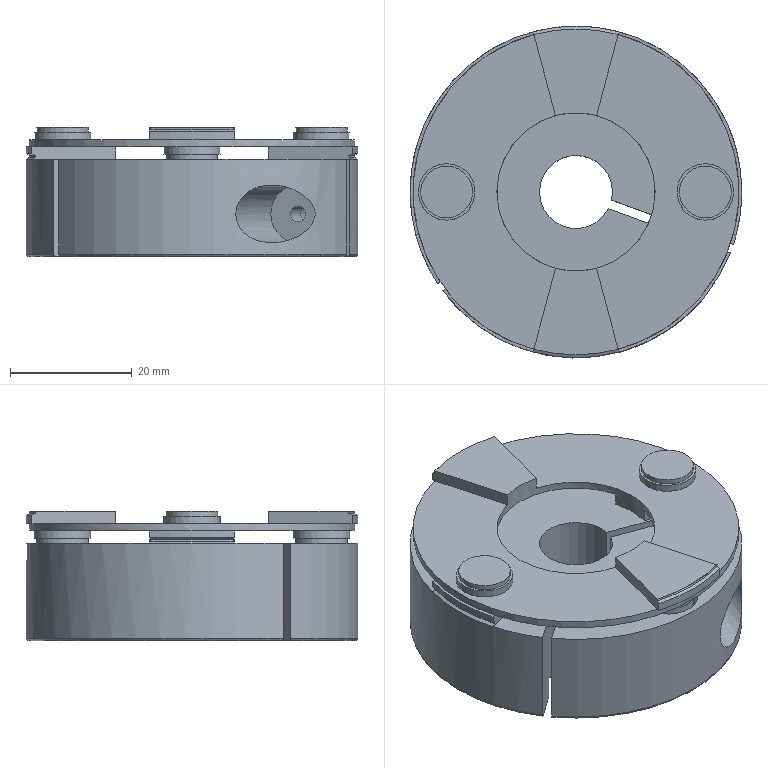Part | NX | features L_5003_007_C-SCPW55-12-15 2 | 1 solid | 84 faces | box 54.5 x 54.5 x 21.2 mm | volume 35031 mm3 | plane 47 | cylinder 23 | cone 8 | torus 6 | commonest cylinder face diameters 54.5 x6 8.5 x4 9.3 x4 10 x2 2.6 x1 4.134 x1